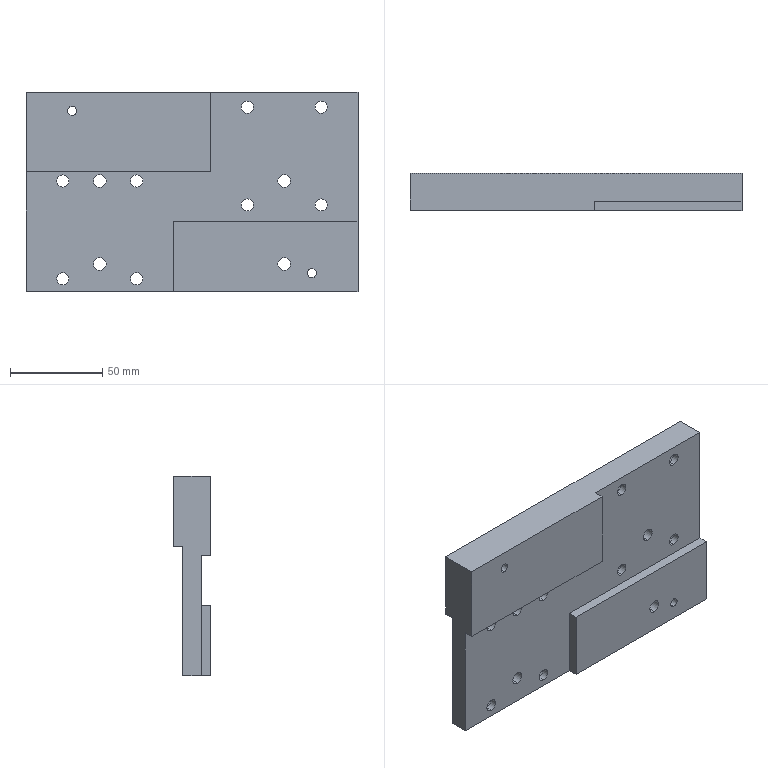Part | STEP file | slider fixing plate | 1 solid | 66 faces | box 180 x 20 x 108 mm | volume 259977 mm3 | cylinder 44 | plane 22 | commonest cylinder face diameters 6.6 x16 11 x16 6.8 x8 5 x4